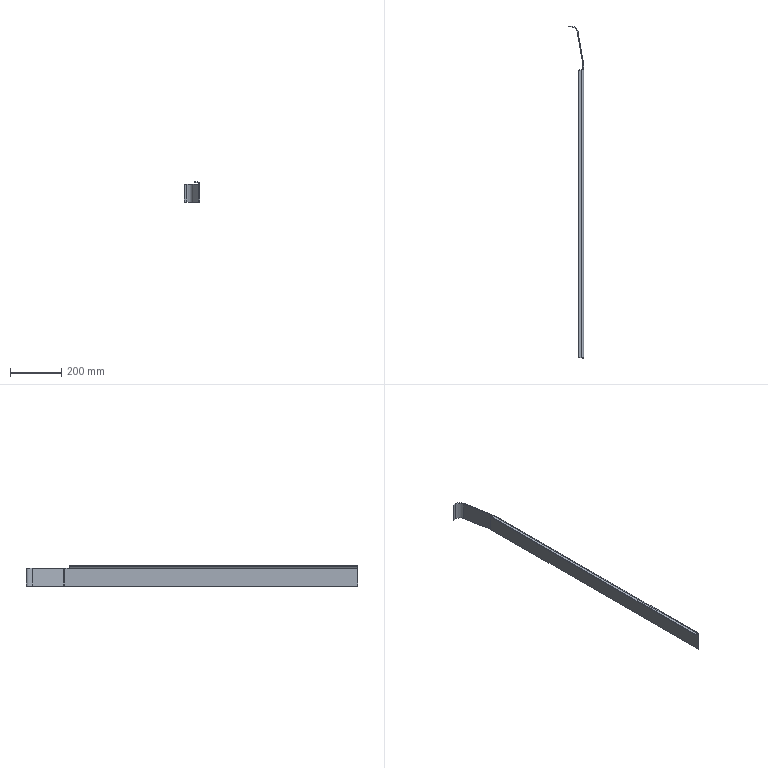Part | SolidWorks | features Fillet 2, EdgeFlange 1, FlatPattern 1, ICE 1, SMBaseFlange 1, SheetMetal 1 | 1 solid | 36 faces | box 60.1 x 1293 x 79 mm | volume 376387 mm3 | plane 26 | cylinder 10 | commonest cylinder face diameters 6 x2 10 x2 50 x2 56.4 x2 12 x1 18.4 x1
STEP:
#1=CARTESIAN_POINT('',(60.2,-1295.7,30.3));
#2=VERTEX_POINT('',#1);
#3=CARTESIAN_POINT('',(60.2,-1295.7,-39.5));
#4=VERTEX_POINT('',#3);
#5=CARTESIAN_POINT('',(60.2,-1295.7,39.5));
#6=DIRECTION('',(0.,0.,-1.));
#7=VECTOR('',#6,1000.);
#8=LINE('',#5,#7);
#9=EDGE_CURVE('',#2,#4,#8,.T.);
#10=ORIENTED_EDGE('',*,*,#9,.F.);
#11=CARTESIAN_POINT('',(60.2,-172.7,30.3));
#12=VERTEX_POINT('',#11);
#13=CARTESIAN_POINT('',(60.2,-172.7,30.3));
#14=DIRECTION('',(0.,-1.,0.));
#15=VECTOR('',#14,1000.);
#16=LINE('',#13,#15);
#17=EDGE_CURVE('',#12,#2,#16,.T.);
#18=ORIENTED_EDGE('',*,*,#17,.F.);
#19=CARTESIAN_POINT('',(60.2,-169.7,27.3));
#20=VERTEX_POINT('',#19);
#21=CARTESIAN_POINT('',(60.2,-169.7,30.3));
#22=DIRECTION('',(1.,0.,0.));
#23=DIRECTION('',(0.,-1.,0.));
#24=AXIS2_PLACEMENT_3D('',#21,#22,#23);
#25=CIRCLE('',#24,3.);
#26=EDGE_CURVE('',#12,#20,#25,.T.);
#27=ORIENTED_EDGE('',*,*,#26,.T.);
#28=CARTESIAN_POINT('',(60.2,-166.7,30.3));
#29=VERTEX_POINT('',#28);
#30=CARTESIAN_POINT('',(60.2,-169.7,30.3));
#31=DIRECTION('',(1.,0.,0.));
#32=DIRECTION('',(0.,-1.,0.));
#33=AXIS2_PLACEMENT_3D('',#30,#31,#32);
#34=CIRCLE('',#33,3.);
#35=EDGE_CURVE('',#20,#29,#34,.T.);
#36=ORIENTED_EDGE('',*,*,#35,.T.);
#37=CARTESIAN_POINT('',(60.2,-166.7,30.5));
#38=VERTEX_POINT('',#37);
#39=CARTESIAN_POINT('',(60.2,-166.7,39.5));
#40=DIRECTION('',(0.,0.,-1.));
#41=VECTOR('',#40,1000.);
#42=LINE('',#39,#41);
#43=EDGE_CURVE('',#38,#29,#42,.T.);
#44=ORIENTED_EDGE('',*,*,#43,.F.);
#45=CARTESIAN_POINT('',(60.2,-153.273,30.5));
#46=VERTEX_POINT('',#45);
#47=CARTESIAN_POINT('',(60.2,-153.273,30.5));
#48=DIRECTION('',(0.,-1.,0.));
#49=VECTOR('',#48,1000.);
#50=LINE('',#47,#49);
#51=EDGE_CURVE('',#46,#38,#50,.T.);
#52=ORIENTED_EDGE('',*,*,#51,.F.);
#53=CARTESIAN_POINT('',(60.2,-153.273,-39.5));
#54=VERTEX_POINT('',#53);
#55=CARTESIAN_POINT('',(60.2,-153.273,39.5));
#56=DIRECTION('',(0.,0.,-1.));
#57=VECTOR('',#56,1000.);
#58=LINE('',#55,#57);
#59=EDGE_CURVE('',#46,#54,#58,.T.);
#60=ORIENTED_EDGE('',*,*,#59,.T.);
#61=CARTESIAN_POINT('',(60.2,-153.273,-39.5));
#62=DIRECTION('',(0.,1.,0.));
#63=VECTOR('',#62,1000.);
#64=LINE('',#61,#63);
#65=EDGE_CURVE('',#4,#54,#64,.T.);
#66=ORIENTED_EDGE('',*,*,#65,.F.);
#67=EDGE_LOOP('',(#10,#18,#27,#36,#44,#52,#60,#66));
#68=FACE_OUTER_BOUND('',#67,.T.);
#69=CARTESIAN_POINT('',(60.2,-153.273,39.5));
#70=DIRECTION('',(-1.,0.,0.));
#71=DIRECTION('',(0.,-1.,0.));
#72=AXIS2_PLACEMENT_3D('',#69,#70,#71);
#73=PLANE('',#72);
#74=ADVANCED_FACE('',(#68),#73,.T.);
#75=CARTESIAN_POINT('',(63.4,-172.7,30.3));
#76=VERTEX_POINT('',#75);
#77=CARTESIAN_POINT('',(63.4,-1295.7,30.3));
#78=VERTEX_POINT('',#77);
#79=CARTESIAN_POINT('',(63.4,-172.7,30.3));
#80=DIRECTION('',(0.,-1.,0.));
#81=VECTOR('',#80,1000.);
#82=LINE('',#79,#81);
#83=EDGE_CURVE('',#76,#78,#82,.T.);
#84=ORIENTED_EDGE('',*,*,#83,.T.);
#85=CARTESIAN_POINT('',(63.4,-1295.7,-39.5));
#86=VERTEX_POINT('',#85);
#87=CARTESIAN_POINT('',(63.4,-1295.7,39.5));
#88=DIRECTION('',(0.,0.,-1.));
#89=VECTOR('',#88,1000.);
#90=LINE('',#87,#89);
#91=EDGE_CURVE('',#78,#86,#90,.T.);
#92=ORIENTED_EDGE('',*,*,#91,.T.);
#93=CARTESIAN_POINT('',(63.4,-153.273,-39.5));
#94=VERTEX_POINT('',#93);
#95=CARTESIAN_POINT('',(63.4,-153.273,-39.5));
#96=DIRECTION('',(0.,1.,0.));
#97=VECTOR('',#96,1000.);
#98=LINE('',#95,#97);
#99=EDGE_CURVE('',#86,#94,#98,.T.);
#100=ORIENTED_EDGE('',*,*,#99,.T.);
#101=CARTESIAN_POINT('',(63.4,-153.273,30.5));
#102=VERTEX_POINT('',#101);
#103=CARTESIAN_POINT('',(63.4,-153.273,39.5));
#104=DIRECTION('',(0.,0.,-1.));
#105=VECTOR('',#104,1000.);
#106=LINE('',#103,#105);
#107=EDGE_CURVE('',#102,#94,#106,.T.);
#108=ORIENTED_EDGE('',*,*,#107,.F.);
#109=CARTESIAN_POINT('',(63.4,-166.7,30.5));
#110=VERTEX_POINT('',#109);
#111=CARTESIAN_POINT('',(63.4,-2.3,30.5));
#112=DIRECTION('',(0.,1.,0.));
#113=VECTOR('',#112,1000.);
#114=LINE('',#111,#113);
#115=EDGE_CURVE('',#110,#102,#114,.T.);
#116=ORIENTED_EDGE('',*,*,#115,.F.);
#117=CARTESIAN_POINT('',(63.4,-166.7,30.3));
#118=VERTEX_POINT('',#117);
#119=CARTESIAN_POINT('',(63.4,-166.7,30.5));
#120=DIRECTION('',(0.,0.,1.));
#121=VECTOR('',#120,1000.);
#122=LINE('',#119,#121);
#123=EDGE_CURVE('',#118,#110,#122,.T.);
#124=ORIENTED_EDGE('',*,*,#123,.F.);
#125=CARTESIAN_POINT('',(63.4,-169.7,27.3));
#126=VERTEX_POINT('',#125);
#127=CARTESIAN_POINT('',(63.4,-169.7,30.3));
#128=DIRECTION('',(-1.,0.,0.));
#129=DIRECTION('',(0.,-1.,0.));
#130=AXIS2_PLACEMENT_3D('',#127,#128,#129);
#131=CIRCLE('',#130,3.);
#132=EDGE_CURVE('',#118,#126,#131,.T.);
#133=ORIENTED_EDGE('',*,*,#132,.T.);
#134=CARTESIAN_POINT('',(63.4,-169.7,30.3));
#135=DIRECTION('',(-1.,0.,0.));
#136=DIRECTION('',(0.,-1.,0.));
#137=AXIS2_PLACEMENT_3D('',#134,#135,#136);
#138=CIRCLE('',#137,3.);
#139=EDGE_CURVE('',#126,#76,#138,.T.);
#140=ORIENTED_EDGE('',*,*,#139,.T.);
#141=EDGE_LOOP('',(#84,#92,#100,#108,#116,#124,#133,#140));
#142=FACE_OUTER_BOUND('',#141,.T.);
#143=CARTESIAN_POINT('',(63.4,-153.273,39.5));
#144=DIRECTION('',(-1.,0.,0.));
#145=DIRECTION('',(0.,-1.,0.));
#146=AXIS2_PLACEMENT_3D('',#143,#144,#145);
#147=PLANE('',#146);
#148=ADVANCED_FACE('',(#142),#147,.F.);
#149=ORIENTED_EDGE('',*,*,#115,.T.);
#150=CARTESIAN_POINT('',(63.4,-153.273,30.5));
#151=DIRECTION('',(-1.,0.,0.));
#152=VECTOR('',#151,1000.);
#153=LINE('',#150,#152);
#154=EDGE_CURVE('',#102,#46,#153,.T.);
#155=ORIENTED_EDGE('',*,*,#154,.T.);
#156=ORIENTED_EDGE('',*,*,#51,.T.);
#157=CARTESIAN_POINT('',(3.3,-166.7,30.5));
#158=DIRECTION('',(1.,0.,0.));
#159=VECTOR('',#158,1000.);
#160=LINE('',#157,#159);
#161=EDGE_CURVE('',#38,#110,#160,.T.);
#162=ORIENTED_EDGE('',*,*,#161,.T.);
#163=EDGE_LOOP('',(#149,#155,#156,#162));
#164=FACE_OUTER_BOUND('',#163,.T.);
#165=CARTESIAN_POINT('',(3.3,-2.3,30.5));
#166=DIRECTION('',(0.,0.,-1.));
#167=DIRECTION('',(0.,1.,0.));
#168=AXIS2_PLACEMENT_3D('',#165,#166,#167);
#169=PLANE('',#168);
#170=ADVANCED_FACE('',(#164),#169,.F.);
#171=CARTESIAN_POINT('',(38.134,-26.152,30.5));
#172=VERTEX_POINT('',#171);
#173=CARTESIAN_POINT('',(59.819,-148.925,30.5));
#174=VERTEX_POINT('',#173);
#175=CARTESIAN_POINT('',(38.134,-26.152,30.5));
#176=DIRECTION('',(0.1739,-0.9848,0.));
#177=VECTOR('',#176,1000.);
#178=LINE('',#175,#177);
#179=EDGE_CURVE('',#172,#174,#178,.T.);
#180=ORIENTED_EDGE('',*,*,#179,.T.);
#181=CARTESIAN_POINT('',(62.97,-148.368,30.5));
#182=VERTEX_POINT('',#181);
#183=CARTESIAN_POINT('',(59.819,-148.925,30.5));
#184=DIRECTION('',(0.9848,0.1739,0.));
#185=VECTOR('',#184,1000.);
#186=LINE('',#183,#185);
#187=EDGE_CURVE('',#174,#182,#186,.T.);
#188=ORIENTED_EDGE('',*,*,#187,.T.);
#189=CARTESIAN_POINT('',(41.285,-25.595,30.5));
#190=VERTEX_POINT('',#189);
#191=CARTESIAN_POINT('',(41.285,-25.595,30.5));
#192=DIRECTION('',(0.1739,-0.9848,0.));
#193=VECTOR('',#192,1000.);
#194=LINE('',#191,#193);
#195=EDGE_CURVE('',#190,#182,#194,.T.);
#196=ORIENTED_EDGE('',*,*,#195,.F.);
#197=CARTESIAN_POINT('',(41.285,-25.595,30.5));
#198=DIRECTION('',(-0.9848,-0.1739,0.));
#199=VECTOR('',#198,1000.);
#200=LINE('',#197,#199);
#201=EDGE_CURVE('',#190,#172,#200,.T.);
#202=ORIENTED_EDGE('',*,*,#201,.T.);
#203=EDGE_LOOP('',(#180,#188,#196,#202));
#204=FACE_OUTER_BOUND('',#203,.T.);
#205=CARTESIAN_POINT('',(3.3,-2.3,30.5));
#206=DIRECTION('',(0.,0.,-1.));
#207=DIRECTION('',(0.,1.,0.));
#208=AXIS2_PLACEMENT_3D('',#205,#206,#207);
#209=PLANE('',#208);
#210=ADVANCED_FACE('',(#204),#209,.F.);
#211=ORIENTED_EDGE('',*,*,#154,.F.);
#212=CARTESIAN_POINT('',(35.2,-153.273,30.5));
#213=DIRECTION('',(0.,0.,-1.));
#214=DIRECTION('',(0.,1.,0.));
#215=AXIS2_PLACEMENT_3D('',#212,#213,#214);
#216=CIRCLE('',#215,28.2);
#217=EDGE_CURVE('',#182,#102,#216,.T.);
#218=ORIENTED_EDGE('',*,*,#217,.F.);
#219=ORIENTED_EDGE('',*,*,#187,.F.);
#220=CARTESIAN_POINT('',(35.2,-153.273,30.5));
#221=DIRECTION('',(0.,0.,-1.));
#222=DIRECTION('',(0.,1.,0.));
#223=AXIS2_PLACEMENT_3D('',#220,#221,#222);
#224=CIRCLE('',#223,25.);
#225=EDGE_CURVE('',#174,#46,#224,.T.);
#226=ORIENTED_EDGE('',*,*,#225,.T.);
#227=EDGE_LOOP('',(#211,#218,#219,#226));
#228=FACE_OUTER_BOUND('',#227,.T.);
#229=CARTESIAN_POINT('',(3.3,-2.3,30.5));
#230=DIRECTION('',(0.,0.,-1.));
#231=DIRECTION('',(0.,1.,0.));
#232=AXIS2_PLACEMENT_3D('',#229,#230,#231);
#233=PLANE('',#232);
#234=ADVANCED_FACE('',(#228),#233,.F.);
#235=CARTESIAN_POINT('',(3.3,-5.5,30.5));
#236=VERTEX_POINT('',#235);
#237=CARTESIAN_POINT('',(13.515,-5.5,30.5));
#238=VERTEX_POINT('',#237);
#239=CARTESIAN_POINT('',(13.515,-5.5,30.5));
#240=DIRECTION('',(1.,0.,0.));
#241=VECTOR('',#240,1000.);
#242=LINE('',#239,#241);
#243=EDGE_CURVE('',#236,#238,#242,.T.);
#244=ORIENTED_EDGE('',*,*,#243,.T.);
#245=CARTESIAN_POINT('',(13.515,-2.3,30.5));
#246=VERTEX_POINT('',#245);
#247=CARTESIAN_POINT('',(13.515,-5.5,30.5));
#248=DIRECTION('',(0.,1.,0.));
#249=VECTOR('',#248,1000.);
#250=LINE('',#247,#249);
#251=EDGE_CURVE('',#238,#246,#250,.T.);
#252=ORIENTED_EDGE('',*,*,#251,.T.);
#253=CARTESIAN_POINT('',(3.3,-2.3,30.5));
#254=VERTEX_POINT('',#253);
#255=CARTESIAN_POINT('',(3.3,-2.3,30.5));
#256=DIRECTION('',(1.,0.,0.));
#257=VECTOR('',#256,1000.);
#258=LINE('',#255,#257);
#259=EDGE_CURVE('',#254,#246,#258,.T.);
#260=ORIENTED_EDGE('',*,*,#259,.F.);
#261=CARTESIAN_POINT('',(3.3,-2.3,30.5));
#262=DIRECTION('',(0.,1.,0.));
#263=VECTOR('',#262,1000.);
#264=LINE('',#261,#263);
#265=EDGE_CURVE('',#236,#254,#264,.T.);
#266=ORIENTED_EDGE('',*,*,#265,.F.);
#267=EDGE_LOOP('',(#244,#252,#260,#266));
#268=FACE_OUTER_BOUND('',#267,.T.);
#269=CARTESIAN_POINT('',(3.3,-2.3,30.5));
#270=DIRECTION('',(0.,0.,-1.));
#271=DIRECTION('',(0.,1.,0.));
#272=AXIS2_PLACEMENT_3D('',#269,#270,#271);
#273=PLANE('',#272);
#274=ADVANCED_FACE('',(#268),#273,.F.);
#275=CARTESIAN_POINT('',(60.2,-153.273,-39.5));
#276=DIRECTION('',(1.,0.,0.));
#277=VECTOR('',#276,1000.);
#278=LINE('',#275,#277);
#279=EDGE_CURVE('',#54,#94,#278,.T.);
#280=ORIENTED_EDGE('',*,*,#279,.F.);
#281=CARTESIAN_POINT('',(59.819,-148.925,-39.5));
#282=VERTEX_POINT('',#281);
#283=CARTESIAN_POINT('',(35.2,-153.273,-39.5));
#284=DIRECTION('',(0.,0.,1.));
#285=DIRECTION('',(-1.,0.,0.));
#286=AXIS2_PLACEMENT_3D('',#283,#284,#285);
#287=CIRCLE('',#286,25.);
#288=EDGE_CURVE('',#54,#282,#287,.T.);
#289=ORIENTED_EDGE('',*,*,#288,.T.);
#290=CARTESIAN_POINT('',(62.97,-148.368,-39.5));
#291=VERTEX_POINT('',#290);
#292=CARTESIAN_POINT('',(62.97,-148.368,-39.5));
#293=DIRECTION('',(-0.9848,-0.1739,0.));
#294=VECTOR('',#293,1000.);
#295=LINE('',#292,#294);
#296=EDGE_CURVE('',#291,#282,#295,.T.);
#297=ORIENTED_EDGE('',*,*,#296,.F.);
#298=CARTESIAN_POINT('',(35.2,-153.273,-39.5));
#299=DIRECTION('',(0.,0.,1.));
#300=DIRECTION('',(1.,0.,0.));
#301=AXIS2_PLACEMENT_3D('',#298,#299,#300);
#302=CIRCLE('',#301,28.2);
#303=EDGE_CURVE('',#94,#291,#302,.T.);
#304=ORIENTED_EDGE('',*,*,#303,.F.);
#305=EDGE_LOOP('',(#280,#289,#297,#304));
#306=FACE_OUTER_BOUND('',#305,.T.);
#307=CARTESIAN_POINT('',(60.2,-153.273,-39.5));
#308=DIRECTION('',(0.,0.,-1.));
#309=DIRECTION('',(-1.,0.,0.));
#310=AXIS2_PLACEMENT_3D('',#307,#308,#309);
#311=PLANE('',#310);
#312=ADVANCED_FACE('',(#306),#311,.T.);
#313=ORIENTED_EDGE('',*,*,#65,.T.);
#314=ORIENTED_EDGE('',*,*,#279,.T.);
#315=ORIENTED_EDGE('',*,*,#99,.F.);
#316=CARTESIAN_POINT('',(63.4,-1295.7,-39.5));
#317=DIRECTION('',(-1.,0.,0.));
#318=VECTOR('',#317,1000.);
#319=LINE('',#316,#318);
#320=EDGE_CURVE('',#86,#4,#319,.T.);
#321=ORIENTED_EDGE('',*,*,#320,.T.);
#322=EDGE_LOOP('',(#313,#314,#315,#321));
#323=FACE_OUTER_BOUND('',#322,.T.);
#324=CARTESIAN_POINT('',(62.97,-148.368,-39.5));
#325=DIRECTION('',(0.,0.,-1.));
#326=DIRECTION('',(-1.,0.,0.));
#327=AXIS2_PLACEMENT_3D('',#324,#325,#326);
#328=PLANE('',#327);
#329=ADVANCED_FACE('',(#323),#328,.T.);
#330=CARTESIAN_POINT('',(38.134,-26.152,-39.5));
#331=VERTEX_POINT('',#330);
#332=CARTESIAN_POINT('',(41.285,-25.595,-39.5));
#333=VERTEX_POINT('',#332);
#334=CARTESIAN_POINT('',(38.134,-26.152,-39.5));
#335=DIRECTION('',(0.9848,0.1739,0.));
#336=VECTOR('',#335,1000.);
#337=LINE('',#334,#336);
#338=EDGE_CURVE('',#331,#333,#337,.T.);
#339=ORIENTED_EDGE('',*,*,#338,.F.);
#340=CARTESIAN_POINT('',(13.515,-5.5,-39.5));
#341=VERTEX_POINT('',#340);
#342=CARTESIAN_POINT('',(13.515,-30.5,-39.5));
#343=DIRECTION('',(0.,0.,1.));
#344=DIRECTION('',(-1.,0.,0.));
#345=AXIS2_PLACEMENT_3D('',#342,#343,#344);
#346=CIRCLE('',#345,25.);
#347=EDGE_CURVE('',#331,#341,#346,.T.);
#348=ORIENTED_EDGE('',*,*,#347,.T.);
#349=CARTESIAN_POINT('',(13.515,-2.3,-39.5));
#350=VERTEX_POINT('',#349);
#351=CARTESIAN_POINT('',(13.515,-2.3,-39.5));
#352=DIRECTION('',(0.,-1.,0.));
#353=VECTOR('',#352,1000.);
#354=LINE('',#351,#353);
#355=EDGE_CURVE('',#350,#341,#354,.T.);
#356=ORIENTED_EDGE('',*,*,#355,.F.);
#357=CARTESIAN_POINT('',(13.515,-30.5,-39.5));
#358=DIRECTION('',(0.,0.,1.));
#359=DIRECTION('',(1.,0.,0.));
#360=AXIS2_PLACEMENT_3D('',#357,#358,#359);
#361=CIRCLE('',#360,28.2);
#362=EDGE_CURVE('',#333,#350,#361,.T.);
#363=ORIENTED_EDGE('',*,*,#362,.F.);
#364=EDGE_LOOP('',(#339,#348,#356,#363));
#365=FACE_OUTER_BOUND('',#364,.T.);
#366=CARTESIAN_POINT('',(38.134,-26.152,-39.5));
#367=DIRECTION('',(0.,0.,-1.));
#368=DIRECTION('',(-1.,0.,0.));
#369=AXIS2_PLACEMENT_3D('',#366,#367,#368);
#370=PLANE('',#369);
#371=ADVANCED_FACE('',(#365),#370,.T.);
#372=CARTESIAN_POINT('',(38.134,-26.152,-39.5));
#373=DIRECTION('',(-0.1739,0.9848,0.));
#374=VECTOR('',#373,1000.);
#375=LINE('',#372,#374);
#376=EDGE_CURVE('',#282,#331,#375,.T.);
#377=ORIENTED_EDGE('',*,*,#376,.T.);
#378=ORIENTED_EDGE('',*,*,#338,.T.);
#379=CARTESIAN_POINT('',(41.285,-25.595,-39.5));
#380=DIRECTION('',(-0.1739,0.9848,0.));
#381=VECTOR('',#380,1000.);
#382=LINE('',#379,#381);
#383=EDGE_CURVE('',#291,#333,#382,.T.);
#384=ORIENTED_EDGE('',*,*,#383,.F.);
#385=ORIENTED_EDGE('',*,*,#296,.T.);
#386=EDGE_LOOP('',(#377,#378,#384,#385));
#387=FACE_OUTER_BOUND('',#386,.T.);
#388=CARTESIAN_POINT('',(13.515,-2.3,-39.5));
#389=DIRECTION('',(0.,0.,-1.));
#390=DIRECTION('',(-1.,0.,0.));
#391=AXIS2_PLACEMENT_3D('',#388,#389,#390);
#392=PLANE('',#391);
#393=ADVANCED_FACE('',(#387),#392,.T.);
#394=CARTESIAN_POINT('',(3.3,-2.3,-39.5));
#395=VERTEX_POINT('',#394);
#396=CARTESIAN_POINT('',(3.3,-2.3,39.5));
#397=DIRECTION('',(0.,0.,-1.));
#398=VECTOR('',#397,1000.);
#399=LINE('',#396,#398);
#400=EDGE_CURVE('',#254,#395,#399,.T.);
#401=ORIENTED_EDGE('',*,*,#400,.F.);
#402=ORIENTED_EDGE('',*,*,#259,.T.);
#403=CARTESIAN_POINT('',(13.515,-2.3,39.5));
#404=DIRECTION('',(0.,0.,-1.));
#405=VECTOR('',#404,1000.);
#406=LINE('',#403,#405);
#407=EDGE_CURVE('',#246,#350,#406,.T.);
#408=ORIENTED_EDGE('',*,*,#407,.T.);
#409=CARTESIAN_POINT('',(13.515,-2.3,-39.5));
#410=DIRECTION('',(-1.,0.,0.));
#411=VECTOR('',#410,1000.);
#412=LINE('',#409,#411);
#413=EDGE_CURVE('',#350,#395,#412,.T.);
#414=ORIENTED_EDGE('',*,*,#413,.T.);
#415=EDGE_LOOP('',(#401,#402,#408,#414));
#416=FACE_OUTER_BOUND('',#415,.T.);
#417=CARTESIAN_POINT('',(13.515,-2.3,39.5));
#418=DIRECTION('',(0.,-1.,0.));
#419=DIRECTION('',(1.,0.,0.));
#420=AXIS2_PLACEMENT_3D('',#417,#418,#419);
#421=PLANE('',#420);
#422=ADVANCED_FACE('',(#416),#421,.F.);
#423=ORIENTED_EDGE('',*,*,#265,.T.);
#424=ORIENTED_EDGE('',*,*,#400,.T.);
#425=CARTESIAN_POINT('',(3.3,-5.5,-39.5));
#426=VERTEX_POINT('',#425);
#427=CARTESIAN_POINT('',(3.3,-5.5,-39.5));
#428=DIRECTION('',(0.,1.,0.));
#429=VECTOR('',#428,1000.);
#430=LINE('',#427,#429);
#431=EDGE_CURVE('',#426,#395,#430,.T.);
#432=ORIENTED_EDGE('',*,*,#431,.F.);
#433=CARTESIAN_POINT('',(3.3,-5.5,39.5));
#434=DIRECTION('',(0.,0.,-1.));
#435=VECTOR('',#434,1000.);
#436=LINE('',#433,#435);
#437=EDGE_CURVE('',#236,#426,#436,.T.);
#438=ORIENTED_EDGE('',*,*,#437,.F.);
#439=EDGE_LOOP('',(#423,#424,#432,#438));
#440=FACE_OUTER_BOUND('',#439,.T.);
#441=CARTESIAN_POINT('',(3.3,-5.5,39.5));
#442=DIRECTION('',(-1.,0.,0.));
#443=DIRECTION('',(0.,-1.,0.));
#444=AXIS2_PLACEMENT_3D('',#441,#442,#443);
#445=PLANE('',#444);
#446=ADVANCED_FACE('',(#440),#445,.T.);
#447=ORIENTED_EDGE('',*,*,#243,.F.);
#448=ORIENTED_EDGE('',*,*,#437,.T.);
#449=CARTESIAN_POINT('',(13.515,-5.5,-39.5));
#450=DIRECTION('',(-1.,0.,0.));
#451=VECTOR('',#450,1000.);
#452=LINE('',#449,#451);
#453=EDGE_CURVE('',#341,#426,#452,.T.);
#454=ORIENTED_EDGE('',*,*,#453,.F.);
#455=CARTESIAN_POINT('',(13.515,-5.5,39.5));
#456=DIRECTION('',(0.,0.,-1.));
#457=VECTOR('',#456,1000.);
#458=LINE('',#455,#457);
#459=EDGE_CURVE('',#238,#341,#458,.T.);
#460=ORIENTED_EDGE('',*,*,#459,.F.);
#461=EDGE_LOOP('',(#447,#448,#454,#460));
#462=FACE_OUTER_BOUND('',#461,.T.);
#463=CARTESIAN_POINT('',(13.515,-5.5,39.5));
#464=DIRECTION('',(0.,-1.,0.));
#465=DIRECTION('',(1.,0.,0.));
#466=AXIS2_PLACEMENT_3D('',#463,#464,#465);
#467=PLANE('',#466);
#468=ADVANCED_FACE('',(#462),#467,.T.);
#469=CARTESIAN_POINT('',(13.515,-30.5,30.5));
#470=DIRECTION('',(0.,0.,-1.));
#471=DIRECTION('',(0.,1.,0.));
#472=AXIS2_PLACEMENT_3D('',#469,#470,#471);
#473=CIRCLE('',#472,25.);
#474=EDGE_CURVE('',#238,#172,#473,.T.);
#475=ORIENTED_EDGE('',*,*,#474,.F.);
#476=ORIENTED_EDGE('',*,*,#459,.T.);
#477=ORIENTED_EDGE('',*,*,#347,.F.);
#478=CARTESIAN_POINT('',(38.134,-26.152,39.5));
#479=DIRECTION('',(0.,0.,-1.));
#480=VECTOR('',#479,1000.);
#481=LINE('',#478,#480);
#482=EDGE_CURVE('',#172,#331,#481,.T.);
#483=ORIENTED_EDGE('',*,*,#482,.F.);
#484=EDGE_LOOP('',(#475,#476,#477,#483));
#485=FACE_OUTER_BOUND('',#484,.T.);
#486=CARTESIAN_POINT('',(13.515,-30.5,39.5));
#487=DIRECTION('',(0.,0.,-1.));
#488=DIRECTION('',(-1.,0.,0.));
#489=AXIS2_PLACEMENT_3D('',#486,#487,#488);
#490=CYLINDRICAL_SURFACE('',#489,25.);
#491=ADVANCED_FACE('',(#485),#490,.F.);
#492=ORIENTED_EDGE('',*,*,#179,.F.);
#493=ORIENTED_EDGE('',*,*,#482,.T.);
#494=ORIENTED_EDGE('',*,*,#376,.F.);
#495=CARTESIAN_POINT('',(59.819,-148.925,39.5));
#496=DIRECTION('',(0.,0.,-1.));
#497=VECTOR('',#496,1000.);
#498=LINE('',#495,#497);
#499=EDGE_CURVE('',#174,#282,#498,.T.);
#500=ORIENTED_EDGE('',*,*,#499,.F.);
#501=EDGE_LOOP('',(#492,#493,#494,#500));
#502=FACE_OUTER_BOUND('',#501,.T.);
#503=CARTESIAN_POINT('',(38.134,-26.152,39.5));
#504=DIRECTION('',(-0.9848,-0.1739,0.));
#505=DIRECTION('',(0.1739,-0.9848,0.));
#506=AXIS2_PLACEMENT_3D('',#503,#504,#505);
#507=PLANE('',#506);
#508=ADVANCED_FACE('',(#502),#507,.T.);
#509=ORIENTED_EDGE('',*,*,#225,.F.);
#510=ORIENTED_EDGE('',*,*,#499,.T.);
#511=ORIENTED_EDGE('',*,*,#288,.F.);
#512=ORIENTED_EDGE('',*,*,#59,.F.);
#513=EDGE_LOOP('',(#509,#510,#511,#512));
#514=FACE_OUTER_BOUND('',#513,.T.);
#515=CARTESIAN_POINT('',(35.2,-153.273,39.5));
#516=DIRECTION('',(0.,0.,-1.));
#517=DIRECTION('',(-1.,0.,0.));
#518=AXIS2_PLACEMENT_3D('',#515,#516,#517);
#519=CYLINDRICAL_SURFACE('',#518,25.);
#520=ADVANCED_FACE('',(#514),#519,.F.);
#521=CARTESIAN_POINT('',(60.2,-1295.7,30.3));
#522=DIRECTION('',(1.,0.,0.));
#523=VECTOR('',#522,1000.);
#524=LINE('',#521,#523);
#525=EDGE_CURVE('',#2,#78,#524,.T.);
#526=ORIENTED_EDGE('',*,*,#525,.F.);
#527=ORIENTED_EDGE('',*,*,#9,.T.);
#528=ORIENTED_EDGE('',*,*,#320,.F.);
#529=ORIENTED_EDGE('',*,*,#91,.F.);
#530=EDGE_LOOP('',(#526,#527,#528,#529));
#531=FACE_OUTER_BOUND('',#530,.T.);
#532=CARTESIAN_POINT('',(63.4,-1295.7,39.5));
#533=DIRECTION('',(0.,-1.,0.));
#534=DIRECTION('',(0.,0.,-1.));
#535=AXIS2_PLACEMENT_3D('',#532,#533,#534);
#536=PLANE('',#535);
#537=ADVANCED_FACE('',(#531),#536,.T.);
#538=CARTESIAN_POINT('',(62.97,-148.368,39.5));
#539=DIRECTION('',(0.,0.,-1.));
#540=VECTOR('',#539,1000.);
#541=LINE('',#538,#540);
#542=EDGE_CURVE('',#182,#291,#541,.T.);
#543=ORIENTED_EDGE('',*,*,#542,.F.);
#544=ORIENTED_EDGE('',*,*,#217,.T.);
#545=ORIENTED_EDGE('',*,*,#107,.T.);
#546=ORIENTED_EDGE('',*,*,#303,.T.);
#547=EDGE_LOOP('',(#543,#544,#545,#546));
#548=FACE_OUTER_BOUND('',#547,.T.);
#549=CARTESIAN_POINT('',(35.2,-153.273,39.5));
#550=DIRECTION('',(0.,0.,-1.));
#551=DIRECTION('',(-1.,0.,0.));
#552=AXIS2_PLACEMENT_3D('',#549,#550,#551);
#553=CYLINDRICAL_SURFACE('',#552,28.2);
#554=ADVANCED_FACE('',(#548),#553,.T.);
#555=CARTESIAN_POINT('',(41.285,-25.595,39.5));
#556=DIRECTION('',(0.,0.,-1.));
#557=VECTOR('',#556,1000.);
#558=LINE('',#555,#557);
#559=EDGE_CURVE('',#190,#333,#558,.T.);
#560=ORIENTED_EDGE('',*,*,#559,.F.);
#561=ORIENTED_EDGE('',*,*,#195,.T.);
#562=ORIENTED_EDGE('',*,*,#542,.T.);
#563=ORIENTED_EDGE('',*,*,#383,.T.);
#564=EDGE_LOOP('',(#560,#561,#562,#563));
#565=FACE_OUTER_BOUND('',#564,.T.);
#566=CARTESIAN_POINT('',(41.285,-25.595,39.5));
#567=DIRECTION('',(-0.9848,-0.1739,0.));
#568=DIRECTION('',(0.1739,-0.9848,0.));
#569=AXIS2_PLACEMENT_3D('',#566,#567,#568);
#570=PLANE('',#569);
#571=ADVANCED_FACE('',(#565),#570,.F.);
#572=ORIENTED_EDGE('',*,*,#407,.F.);
#573=CARTESIAN_POINT('',(13.515,-30.5,30.5));
#574=DIRECTION('',(0.,0.,-1.));
#575=DIRECTION('',(0.,1.,0.));
#576=AXIS2_PLACEMENT_3D('',#573,#574,#575);
#577=CIRCLE('',#576,28.2);
#578=EDGE_CURVE('',#246,#190,#577,.T.);
#579=ORIENTED_EDGE('',*,*,#578,.T.);
#580=ORIENTED_EDGE('',*,*,#559,.T.);
#581=ORIENTED_EDGE('',*,*,#362,.T.);
#582=EDGE_LOOP('',(#572,#579,#580,#581));
#583=FACE_OUTER_BOUND('',#582,.T.);
#584=CARTESIAN_POINT('',(13.515,-30.5,39.5));
#585=DIRECTION('',(0.,0.,-1.));
#586=DIRECTION('',(-1.,0.,0.));
#587=AXIS2_PLACEMENT_3D('',#584,#585,#586);
#588=CYLINDRICAL_SURFACE('',#587,28.2);
#589=ADVANCED_FACE('',(#583),#588,.T.);
#590=ORIENTED_EDGE('',*,*,#413,.F.);
#591=ORIENTED_EDGE('',*,*,#355,.T.);
#592=ORIENTED_EDGE('',*,*,#453,.T.);
#593=ORIENTED_EDGE('',*,*,#431,.T.);
#594=EDGE_LOOP('',(#590,#591,#592,#593));
#595=FACE_OUTER_BOUND('',#594,.T.);
#596=CARTESIAN_POINT('',(13.515,-30.5,-39.5));
#597=DIRECTION('',(0.,0.,1.));
#598=DIRECTION('',(1.,0.,0.));
#599=AXIS2_PLACEMENT_3D('',#596,#597,#598);
#600=PLANE('',#599);
#601=ADVANCED_FACE('',(#595),#600,.F.);
#602=ORIENTED_EDGE('',*,*,#201,.F.);
#603=ORIENTED_EDGE('',*,*,#578,.F.);
#604=ORIENTED_EDGE('',*,*,#251,.F.);
#605=ORIENTED_EDGE('',*,*,#474,.T.);
#606=EDGE_LOOP('',(#602,#603,#604,#605));
#607=FACE_OUTER_BOUND('',#606,.T.);
#608=CARTESIAN_POINT('',(3.3,-2.3,30.5));
#609=DIRECTION('',(0.,0.,-1.));
#610=DIRECTION('',(0.,1.,0.));
#611=AXIS2_PLACEMENT_3D('',#608,#609,#610);
#612=PLANE('',#611);
#613=ADVANCED_FACE('',(#607),#612,.F.);
#614=ORIENTED_EDGE('',*,*,#43,.T.);
#615=CARTESIAN_POINT('',(63.4,-166.7,30.3));
#616=DIRECTION('',(1.,0.,0.));
#617=VECTOR('',#616,1000.);
#618=LINE('',#615,#617);
#619=EDGE_CURVE('',#29,#118,#618,.T.);
#620=ORIENTED_EDGE('',*,*,#619,.T.);
#621=ORIENTED_EDGE('',*,*,#123,.T.);
#622=ORIENTED_EDGE('',*,*,#161,.F.);
#623=EDGE_LOOP('',(#614,#620,#621,#622));
#624=FACE_OUTER_BOUND('',#623,.T.);
#625=CARTESIAN_POINT('',(3.3,-166.7,30.5));
#626=DIRECTION('',(0.,1.,0.));
#627=DIRECTION('',(-1.,0.,0.));
#628=AXIS2_PLACEMENT_3D('',#625,#626,#627);
#629=PLANE('',#628);
#630=ADVANCED_FACE('',(#624),#629,.F.);
#631=CARTESIAN_POINT('',(54.2,-1295.7,36.3));
#632=VERTEX_POINT('',#631);
#633=CARTESIAN_POINT('',(54.2,-1295.7,39.5));
#634=VERTEX_POINT('',#633);
#635=CARTESIAN_POINT('',(54.2,-1295.7,39.5));
#636=DIRECTION('',(0.,0.,1.));
#637=VECTOR('',#636,1000.);
#638=LINE('',#635,#637);
#639=EDGE_CURVE('',#632,#634,#638,.T.);
#640=ORIENTED_EDGE('',*,*,#639,.F.);
#641=CARTESIAN_POINT('',(54.2,-1295.7,30.3));
#642=DIRECTION('',(0.,-1.,0.));
#643=DIRECTION('',(0.,0.,1.));
#644=AXIS2_PLACEMENT_3D('',#641,#642,#643);
#645=CIRCLE('',#644,6.);
#646=EDGE_CURVE('',#2,#632,#645,.T.);
#647=ORIENTED_EDGE('',*,*,#646,.F.);
#648=ORIENTED_EDGE('',*,*,#525,.T.);
#649=CARTESIAN_POINT('',(54.2,-1295.7,30.3));
#650=DIRECTION('',(0.,-1.,0.));
#651=DIRECTION('',(0.,0.,1.));
#652=AXIS2_PLACEMENT_3D('',#649,#650,#651);
#653=CIRCLE('',#652,9.2);
#654=EDGE_CURVE('',#78,#634,#653,.T.);
#655=ORIENTED_EDGE('',*,*,#654,.T.);
#656=EDGE_LOOP('',(#640,#647,#648,#655));
#657=FACE_OUTER_BOUND('',#656,.T.);
#658=CARTESIAN_POINT('',(54.2,-1295.7,30.3));
#659=DIRECTION('',(0.,-1.,0.));
#660=DIRECTION('',(0.,0.,-1.));
#661=AXIS2_PLACEMENT_3D('',#658,#659,#660);
#662=PLANE('',#661);
#663=ADVANCED_FACE('',(#657),#662,.T.);
#664=CARTESIAN_POINT('',(54.2,-172.7,36.3));
#665=VERTEX_POINT('',#664);
#666=CARTESIAN_POINT('',(54.2,-172.7,30.3));
#667=DIRECTION('',(0.,1.,0.));
#668=DIRECTION('',(0.,0.,1.));
#669=AXIS2_PLACEMENT_3D('',#666,#667,#668);
#670=CIRCLE('',#669,6.);
#671=EDGE_CURVE('',#665,#12,#670,.T.);
#672=ORIENTED_EDGE('',*,*,#671,.F.);
#673=CARTESIAN_POINT('',(54.2,-172.7,39.5));
#674=VERTEX_POINT('',#673);
#675=CARTESIAN_POINT('',(54.2,-172.7,36.3));
#676=DIRECTION('',(0.,0.,1.));
#677=VECTOR('',#676,1000.);
#678=LINE('',#675,#677);
#679=EDGE_CURVE('',#665,#674,#678,.T.);
#680=ORIENTED_EDGE('',*,*,#679,.T.);
#681=CARTESIAN_POINT('',(54.2,-172.7,30.3));
#682=DIRECTION('',(0.,1.,0.));
#683=DIRECTION('',(0.,0.,1.));
#684=AXIS2_PLACEMENT_3D('',#681,#682,#683);
#685=CIRCLE('',#684,9.2);
#686=EDGE_CURVE('',#674,#76,#685,.T.);
#687=ORIENTED_EDGE('',*,*,#686,.T.);
#688=CARTESIAN_POINT('',(60.2,-172.7,30.3));
#689=DIRECTION('',(1.,0.,0.));
#690=VECTOR('',#689,1000.);
#691=LINE('',#688,#690);
#692=EDGE_CURVE('',#12,#76,#691,.T.);
#693=ORIENTED_EDGE('',*,*,#692,.F.);
#694=EDGE_LOOP('',(#672,#680,#687,#693));
#695=FACE_OUTER_BOUND('',#694,.T.);
#696=CARTESIAN_POINT('',(54.2,-172.7,30.3));
#697=DIRECTION('',(0.,-1.,0.));
#698=DIRECTION('',(0.,0.,-1.));
#699=AXIS2_PLACEMENT_3D('',#696,#697,#698);
#700=PLANE('',#699);
#701=ADVANCED_FACE('',(#695),#700,.F.);
#702=ORIENTED_EDGE('',*,*,#83,.F.);
#703=ORIENTED_EDGE('',*,*,#686,.F.);
#704=CARTESIAN_POINT('',(54.2,0.,39.5));
#705=DIRECTION('',(0.,1.,0.));
#706=VECTOR('',#705,1000.);
#707=LINE('',#704,#706);
#708=EDGE_CURVE('',#634,#674,#707,.T.);
#709=ORIENTED_EDGE('',*,*,#708,.F.);
#710=ORIENTED_EDGE('',*,*,#654,.F.);
#711=EDGE_LOOP('',(#702,#703,#709,#710));
#712=FACE_OUTER_BOUND('',#711,.T.);
#713=CARTESIAN_POINT('',(54.2,-172.7,30.3));
#714=DIRECTION('',(0.,1.,0.));
#715=DIRECTION('',(0.,0.,1.));
#716=AXIS2_PLACEMENT_3D('',#713,#714,#715);
#717=CYLINDRICAL_SURFACE('',#716,9.2);
#718=ADVANCED_FACE('',(#712),#717,.T.);
#719=ORIENTED_EDGE('',*,*,#17,.T.);
#720=ORIENTED_EDGE('',*,*,#646,.T.);
#721=CARTESIAN_POINT('',(54.2,-1295.7,36.3));
#722=DIRECTION('',(0.,1.,0.));
#723=VECTOR('',#722,1000.);
#724=LINE('',#721,#723);
#725=EDGE_CURVE('',#632,#665,#724,.T.);
#726=ORIENTED_EDGE('',*,*,#725,.T.);
#727=ORIENTED_EDGE('',*,*,#671,.T.);
#728=EDGE_LOOP('',(#719,#720,#726,#727));
#729=FACE_OUTER_BOUND('',#728,.T.);
#730=CARTESIAN_POINT('',(54.2,-172.7,30.3));
#731=DIRECTION('',(0.,1.,0.));
#732=DIRECTION('',(0.,0.,1.));
#733=AXIS2_PLACEMENT_3D('',#730,#731,#732);
#734=CYLINDRICAL_SURFACE('',#733,6.);
#735=ADVANCED_FACE('',(#729),#734,.F.);
#736=CARTESIAN_POINT('',(48.4,-172.7,36.3));
#737=VERTEX_POINT('',#736);
#738=CARTESIAN_POINT('',(0.,-172.7,36.3));
#739=DIRECTION('',(1.,0.,0.));
#740=VECTOR('',#739,1000.);
#741=LINE('',#738,#740);
#742=EDGE_CURVE('',#737,#665,#741,.T.);
#743=ORIENTED_EDGE('',*,*,#742,.F.);
#744=CARTESIAN_POINT('',(48.4,-172.7,39.5));
#745=VERTEX_POINT('',#744);
#746=CARTESIAN_POINT('',(48.4,-172.7,39.5));
#747=DIRECTION('',(0.,0.,1.));
#748=VECTOR('',#747,1000.);
#749=LINE('',#746,#748);
#750=EDGE_CURVE('',#737,#745,#749,.T.);
#751=ORIENTED_EDGE('',*,*,#750,.T.);
#752=CARTESIAN_POINT('',(60.2,-172.7,39.5));
#753=DIRECTION('',(1.,0.,0.));
#754=VECTOR('',#753,1000.);
#755=LINE('',#752,#754);
#756=EDGE_CURVE('',#745,#674,#755,.T.);
#757=ORIENTED_EDGE('',*,*,#756,.T.);
#758=ORIENTED_EDGE('',*,*,#679,.F.);
#759=EDGE_LOOP('',(#743,#751,#757,#758));
#760=FACE_OUTER_BOUND('',#759,.T.);
#761=CARTESIAN_POINT('',(60.2,-172.7,39.5));
#762=DIRECTION('',(0.,1.,0.));
#763=DIRECTION('',(0.,0.,1.));
#764=AXIS2_PLACEMENT_3D('',#761,#762,#763);
#765=PLANE('',#764);
#766=ADVANCED_FACE('',(#760),#765,.T.);
#767=CARTESIAN_POINT('',(48.4,-1295.7,39.5));
#768=VERTEX_POINT('',#767);
#769=CARTESIAN_POINT('',(43.4,-1295.7,39.5));
#770=DIRECTION('',(-1.,0.,0.));
#771=VECTOR('',#770,1000.);
#772=LINE('',#769,#771);
#773=EDGE_CURVE('',#634,#768,#772,.T.);
#774=ORIENTED_EDGE('',*,*,#773,.T.);
#775=CARTESIAN_POINT('',(48.4,-1295.7,36.3));
#776=VERTEX_POINT('',#775);
#777=CARTESIAN_POINT('',(48.4,-1295.7,39.5));
#778=DIRECTION('',(0.,0.,-1.));
#779=VECTOR('',#778,1000.);
#780=LINE('',#777,#779);
#781=EDGE_CURVE('',#768,#776,#780,.T.);
#782=ORIENTED_EDGE('',*,*,#781,.T.);
#783=CARTESIAN_POINT('',(0.,-1295.7,36.3));
#784=DIRECTION('',(-1.,0.,0.));
#785=VECTOR('',#784,1000.);
#786=LINE('',#783,#785);
#787=EDGE_CURVE('',#632,#776,#786,.T.);
#788=ORIENTED_EDGE('',*,*,#787,.F.);
#789=ORIENTED_EDGE('',*,*,#639,.T.);
#790=EDGE_LOOP('',(#774,#782,#788,#789));
#791=FACE_OUTER_BOUND('',#790,.T.);
#792=CARTESIAN_POINT('',(43.4,-1295.7,39.5));
#793=DIRECTION('',(0.,-1.,0.));
#794=DIRECTION('',(0.,0.,-1.));
#795=AXIS2_PLACEMENT_3D('',#792,#793,#794);
#796=PLANE('',#795);
#797=ADVANCED_FACE('',(#791),#796,.T.);
#798=CARTESIAN_POINT('',(43.4,-1290.7,39.5));
#799=VERTEX_POINT('',#798);
#800=CARTESIAN_POINT('',(43.4,-177.7,39.5));
#801=VERTEX_POINT('',#800);
#802=CARTESIAN_POINT('',(43.4,-172.7,39.5));
#803=DIRECTION('',(0.,1.,0.));
#804=VECTOR('',#803,1000.);
#805=LINE('',#802,#804);
#806=EDGE_CURVE('',#799,#801,#805,.T.);
#807=ORIENTED_EDGE('',*,*,#806,.F.);
#808=CARTESIAN_POINT('',(48.4,-1290.7,39.5));
#809=DIRECTION('',(0.,0.,1.));
#810=DIRECTION('',(1.,0.,0.));
#811=AXIS2_PLACEMENT_3D('',#808,#809,#810);
#812=CIRCLE('',#811,5.);
#813=EDGE_CURVE('',#799,#768,#812,.T.);
#814=ORIENTED_EDGE('',*,*,#813,.T.);
#815=ORIENTED_EDGE('',*,*,#773,.F.);
#816=ORIENTED_EDGE('',*,*,#708,.T.);
#817=ORIENTED_EDGE('',*,*,#756,.F.);
#818=CARTESIAN_POINT('',(48.4,-177.7,39.5));
#819=DIRECTION('',(0.,0.,1.));
#820=DIRECTION('',(1.,0.,0.));
#821=AXIS2_PLACEMENT_3D('',#818,#819,#820);
#822=CIRCLE('',#821,5.);
#823=EDGE_CURVE('',#745,#801,#822,.T.);
#824=ORIENTED_EDGE('',*,*,#823,.T.);
#825=EDGE_LOOP('',(#807,#814,#815,#816,#817,#824));
#826=FACE_OUTER_BOUND('',#825,.T.);
#827=CARTESIAN_POINT('',(0.,0.,39.5));
#828=DIRECTION('',(0.,0.,1.));
#829=DIRECTION('',(1.,0.,0.));
#830=AXIS2_PLACEMENT_3D('',#827,#828,#829);
#831=PLANE('',#830);
#832=ADVANCED_FACE('',(#826),#831,.T.);
#833=ORIENTED_EDGE('',*,*,#787,.T.);
#834=CARTESIAN_POINT('',(43.4,-1290.7,36.3));
#835=VERTEX_POINT('',#834);
#836=CARTESIAN_POINT('',(48.4,-1290.7,36.3));
#837=DIRECTION('',(0.,0.,-1.));
#838=DIRECTION('',(1.,0.,0.));
#839=AXIS2_PLACEMENT_3D('',#836,#837,#838);
#840=CIRCLE('',#839,5.);
#841=EDGE_CURVE('',#776,#835,#840,.T.);
#842=ORIENTED_EDGE('',*,*,#841,.T.);
#843=CARTESIAN_POINT('',(43.4,-177.7,36.3));
#844=VERTEX_POINT('',#843);
#845=CARTESIAN_POINT('',(43.4,0.,36.3));
#846=DIRECTION('',(0.,1.,0.));
#847=VECTOR('',#846,1000.);
#848=LINE('',#845,#847);
#849=EDGE_CURVE('',#835,#844,#848,.T.);
#850=ORIENTED_EDGE('',*,*,#849,.T.);
#851=CARTESIAN_POINT('',(48.4,-177.7,36.3));
#852=DIRECTION('',(0.,0.,-1.));
#853=DIRECTION('',(1.,0.,0.));
#854=AXIS2_PLACEMENT_3D('',#851,#852,#853);
#855=CIRCLE('',#854,5.);
#856=EDGE_CURVE('',#844,#737,#855,.T.);
#857=ORIENTED_EDGE('',*,*,#856,.T.);
#858=ORIENTED_EDGE('',*,*,#742,.T.);
#859=ORIENTED_EDGE('',*,*,#725,.F.);
#860=EDGE_LOOP('',(#833,#842,#850,#857,#858,#859));
#861=FACE_OUTER_BOUND('',#860,.T.);
#862=CARTESIAN_POINT('',(0.,0.,36.3));
#863=DIRECTION('',(0.,0.,1.));
#864=DIRECTION('',(1.,0.,0.));
#865=AXIS2_PLACEMENT_3D('',#862,#863,#864);
#866=PLANE('',#865);
#867=ADVANCED_FACE('',(#861),#866,.F.);
#868=ORIENTED_EDGE('',*,*,#849,.F.);
#869=CARTESIAN_POINT('',(43.4,-1290.7,39.5));
#870=DIRECTION('',(0.,0.,1.));
#871=VECTOR('',#870,1000.);
#872=LINE('',#869,#871);
#873=EDGE_CURVE('',#835,#799,#872,.T.);
#874=ORIENTED_EDGE('',*,*,#873,.T.);
#875=ORIENTED_EDGE('',*,*,#806,.T.);
#876=CARTESIAN_POINT('',(43.4,-177.7,39.5));
#877=DIRECTION('',(0.,0.,-1.));
#878=VECTOR('',#877,1000.);
#879=LINE('',#876,#878);
#880=EDGE_CURVE('',#801,#844,#879,.T.);
#881=ORIENTED_EDGE('',*,*,#880,.T.);
#882=EDGE_LOOP('',(#868,#874,#875,#881));
#883=FACE_OUTER_BOUND('',#882,.T.);
#884=CARTESIAN_POINT('',(43.4,-172.7,39.5));
#885=DIRECTION('',(-1.,0.,0.));
#886=DIRECTION('',(0.,0.,1.));
#887=AXIS2_PLACEMENT_3D('',#884,#885,#886);
#888=PLANE('',#887);
#889=ADVANCED_FACE('',(#883),#888,.T.);
#890=ORIENTED_EDGE('',*,*,#813,.F.);
#891=ORIENTED_EDGE('',*,*,#873,.F.);
#892=ORIENTED_EDGE('',*,*,#841,.F.);
#893=ORIENTED_EDGE('',*,*,#781,.F.);
#894=EDGE_LOOP('',(#890,#891,#892,#893));
#895=FACE_OUTER_BOUND('',#894,.T.);
#896=CARTESIAN_POINT('',(48.4,-1290.7,39.5));
#897=DIRECTION('',(0.,0.,-1.));
#898=DIRECTION('',(-1.,0.,0.));
#899=AXIS2_PLACEMENT_3D('',#896,#897,#898);
#900=CYLINDRICAL_SURFACE('',#899,5.);
#901=ADVANCED_FACE('',(#895),#900,.T.);
#902=ORIENTED_EDGE('',*,*,#823,.F.);
#903=ORIENTED_EDGE('',*,*,#750,.F.);
#904=ORIENTED_EDGE('',*,*,#856,.F.);
#905=ORIENTED_EDGE('',*,*,#880,.F.);
#906=EDGE_LOOP('',(#902,#903,#904,#905));
#907=FACE_OUTER_BOUND('',#906,.T.);
#908=CARTESIAN_POINT('',(48.4,-177.7,39.5));
#909=DIRECTION('',(0.,0.,-1.));
#910=DIRECTION('',(-1.,0.,0.));
#911=AXIS2_PLACEMENT_3D('',#908,#909,#910);
#912=CYLINDRICAL_SURFACE('',#911,5.);
#913=ADVANCED_FACE('',(#907),#912,.T.);
#914=CARTESIAN_POINT('',(63.4,-169.7,27.3));
#915=DIRECTION('',(1.,0.,0.));
#916=VECTOR('',#915,1000.);
#917=LINE('',#914,#916);
#918=EDGE_CURVE('',#20,#126,#917,.T.);
#919=ORIENTED_EDGE('',*,*,#918,.F.);
#920=ORIENTED_EDGE('',*,*,#26,.F.);
#921=ORIENTED_EDGE('',*,*,#692,.T.);
#922=ORIENTED_EDGE('',*,*,#139,.F.);
#923=EDGE_LOOP('',(#919,#920,#921,#922));
#924=FACE_OUTER_BOUND('',#923,.T.);
#925=CARTESIAN_POINT('',(3.3,-169.7,30.3));
#926=DIRECTION('',(-1.,0.,0.));
#927=DIRECTION('',(0.,-1.,0.));
#928=AXIS2_PLACEMENT_3D('',#925,#926,#927);
#929=CYLINDRICAL_SURFACE('',#928,3.);
#930=ADVANCED_FACE('',(#924),#929,.F.);
#931=ORIENTED_EDGE('',*,*,#35,.F.);
#932=ORIENTED_EDGE('',*,*,#918,.T.);
#933=ORIENTED_EDGE('',*,*,#132,.F.);
#934=ORIENTED_EDGE('',*,*,#619,.F.);
#935=EDGE_LOOP('',(#931,#932,#933,#934));
#936=FACE_OUTER_BOUND('',#935,.T.);
#937=CARTESIAN_POINT('',(3.3,-169.7,30.3));
#938=DIRECTION('',(-1.,0.,0.));
#939=DIRECTION('',(0.,-1.,0.));
#940=AXIS2_PLACEMENT_3D('',#937,#938,#939);
#941=CYLINDRICAL_SURFACE('',#940,3.);
#942=ADVANCED_FACE('',(#936),#941,.F.);
#943=CLOSED_SHELL('',(#74,#148,#170,#210,#234,#274,#312,#329,#371,#393,#422,#446,#468,#491,#508,#520,#537,#554,#571,#589,#601,#613,#630,#663,#701,#718,#735,#766,#797,#832,#867,#889,#901,#913,#930,#942));
#944=MANIFOLD_SOLID_BREP('',#943);
#945=CARTESIAN_POINT('',(0.,0.,0.));
#946=DIRECTION('',(0.,0.,1.));
#947=DIRECTION('',(1.,0.,0.));
#948=AXIS2_PLACEMENT_3D('',#945,#946,#947);
#949=(LENGTH_UNIT()NAMED_UNIT(*)SI_UNIT(.MILLI.,.METRE.));
#950=UNCERTAINTY_MEASURE_WITH_UNIT(LENGTH_MEASURE(0.00001),#949,'','');
#951=(NAMED_UNIT(*)PLANE_ANGLE_UNIT()SI_UNIT($,.RADIAN.));
#952=(NAMED_UNIT(*)SI_UNIT($,.STERADIAN.)SOLID_ANGLE_UNIT());
#953=(GEOMETRIC_REPRESENTATION_CONTEXT(3)GLOBAL_UNCERTAINTY_ASSIGNED_CONTEXT((#950))GLOBAL_UNIT_ASSIGNED_CONTEXT((#949,#951,#952))REPRESENTATION_CONTEXT('',''));
#954=ADVANCED_BREP_SHAPE_REPRESENTATION('',(#944,#948),#953);